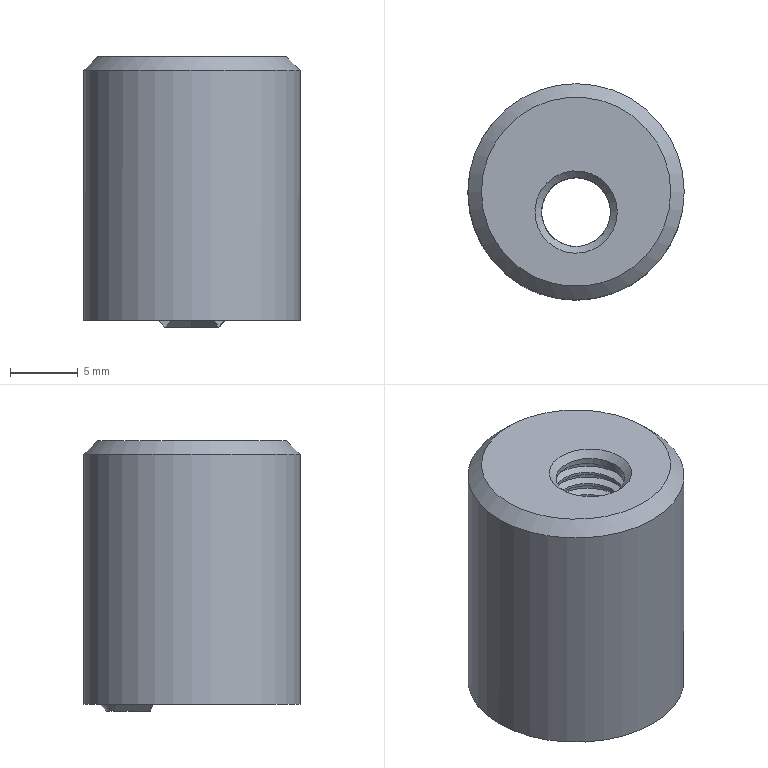Part | NX | features solid 2 | 1 solid | 32 faces | box 16.01 x 16 x 20.005 mm | volume 3045 mm3 | plane 18 | cone 8 | cylinder 4 | spline 2 | commonest cylinder face diameters 5.1 x1 6 x1 9 x1 16 x1